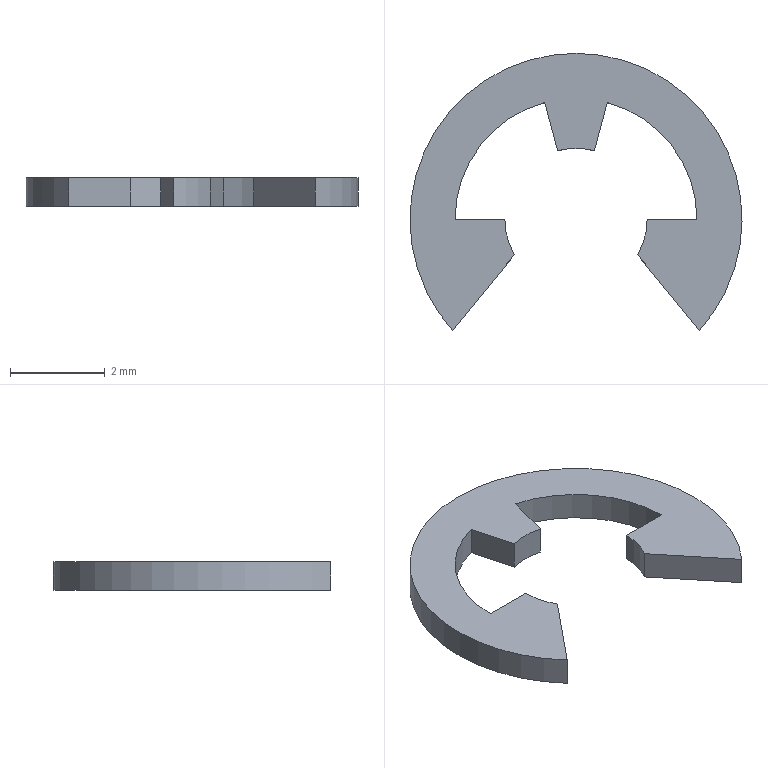Part | NX | 1 solid | 14 faces | box 7 x 5.843 x 0.6 mm | volume 10.111 mm3 | plane 8 | cylinder 6 | commonest cylinder face diameters 3 x3 5.1 x2 7 x1
STEP:
#1=CARTESIAN_POINT('',(2.6,-2.343,-0.3));
#2=VERTEX_POINT('',#1);
#3=CARTESIAN_POINT('',(-2.6,-2.343,-0.3));
#4=VERTEX_POINT('',#3);
#5=CARTESIAN_POINT('',(0.,0.,-0.3));
#6=DIRECTION('',(0.,0.,1.));
#7=DIRECTION('',(0.7429,-0.6694,0.));
#8=AXIS2_PLACEMENT_3D('',#5,#6,#7);
#9=CIRCLE('',#8,3.5);
#10=EDGE_CURVE('',#2,#4,#9,.T.);
#11=ORIENTED_EDGE('',*,*,#10,.T.);
#12=CARTESIAN_POINT('',(-2.6,-2.343,0.3));
#13=VERTEX_POINT('',#12);
#14=CARTESIAN_POINT('',(-2.6,-2.343,0.3));
#15=DIRECTION('',(0.,0.,-1.));
#16=VECTOR('',#15,1000.);
#17=LINE('',#14,#16);
#18=EDGE_CURVE('',#13,#4,#17,.T.);
#19=ORIENTED_EDGE('',*,*,#18,.F.);
#20=CARTESIAN_POINT('',(2.6,-2.343,0.3));
#21=VERTEX_POINT('',#20);
#22=CARTESIAN_POINT('',(0.,0.,0.3));
#23=DIRECTION('',(0.,0.,1.));
#24=DIRECTION('',(0.7429,-0.6694,0.));
#25=AXIS2_PLACEMENT_3D('',#22,#23,#24);
#26=CIRCLE('',#25,3.5);
#27=EDGE_CURVE('',#21,#13,#26,.T.);
#28=ORIENTED_EDGE('',*,*,#27,.F.);
#29=CARTESIAN_POINT('',(2.6,-2.343,0.3));
#30=DIRECTION('',(0.,0.,-1.));
#31=VECTOR('',#30,1000.);
#32=LINE('',#29,#31);
#33=EDGE_CURVE('',#21,#2,#32,.T.);
#34=ORIENTED_EDGE('',*,*,#33,.T.);
#35=EDGE_LOOP('',(#11,#19,#28,#34));
#36=FACE_BOUND('',#35,.T.);
#37=CARTESIAN_POINT('',(0.,0.,0.3));
#38=DIRECTION('',(0.,0.,1.));
#39=DIRECTION('',(0.7429,-0.6694,0.));
#40=AXIS2_PLACEMENT_3D('',#37,#38,#39);
#41=CYLINDRICAL_SURFACE('',#40,3.5);
#42=ADVANCED_FACE('',(#36),#41,.T.);
#43=CARTESIAN_POINT('',(-1.3,-0.7483,-0.3));
#44=VERTEX_POINT('',#43);
#45=CARTESIAN_POINT('',(-2.6,-2.343,-0.3));
#46=DIRECTION('',(0.6318,0.7751,0.));
#47=VECTOR('',#46,1000.);
#48=LINE('',#45,#47);
#49=EDGE_CURVE('',#4,#44,#48,.T.);
#50=ORIENTED_EDGE('',*,*,#49,.T.);
#51=CARTESIAN_POINT('',(-1.3,-0.7483,0.3));
#52=VERTEX_POINT('',#51);
#53=CARTESIAN_POINT('',(-1.3,-0.7483,0.3));
#54=DIRECTION('',(0.,0.,-1.));
#55=VECTOR('',#54,1000.);
#56=LINE('',#53,#55);
#57=EDGE_CURVE('',#52,#44,#56,.T.);
#58=ORIENTED_EDGE('',*,*,#57,.F.);
#59=CARTESIAN_POINT('',(-2.6,-2.343,0.3));
#60=DIRECTION('',(0.6318,0.7751,0.));
#61=VECTOR('',#60,1000.);
#62=LINE('',#59,#61);
#63=EDGE_CURVE('',#13,#52,#62,.T.);
#64=ORIENTED_EDGE('',*,*,#63,.F.);
#65=ORIENTED_EDGE('',*,*,#18,.T.);
#66=EDGE_LOOP('',(#50,#58,#64,#65));
#67=FACE_BOUND('',#66,.T.);
#68=CARTESIAN_POINT('',(-2.6,-2.343,0.3));
#69=DIRECTION('',(0.7751,-0.6318,0.));
#70=DIRECTION('',(0.,0.,-1.));
#71=AXIS2_PLACEMENT_3D('',#68,#69,#70);
#72=PLANE('',#71);
#73=ADVANCED_FACE('',(#67),#72,.T.);
#74=CARTESIAN_POINT('',(-1.5,0.,-0.3));
#75=VERTEX_POINT('',#74);
#76=CARTESIAN_POINT('',(0.,0.,-0.3));
#77=DIRECTION('',(0.,0.,-1.));
#78=DIRECTION('',(-0.8667,-0.4989,0.));
#79=AXIS2_PLACEMENT_3D('',#76,#77,#78);
#80=CIRCLE('',#79,1.5);
#81=EDGE_CURVE('',#44,#75,#80,.T.);
#82=ORIENTED_EDGE('',*,*,#81,.T.);
#83=CARTESIAN_POINT('',(-1.5,0.,0.3));
#84=VERTEX_POINT('',#83);
#85=CARTESIAN_POINT('',(-1.5,0.,0.3));
#86=DIRECTION('',(0.,0.,-1.));
#87=VECTOR('',#86,1000.);
#88=LINE('',#85,#87);
#89=EDGE_CURVE('',#84,#75,#88,.T.);
#90=ORIENTED_EDGE('',*,*,#89,.F.);
#91=CARTESIAN_POINT('',(0.,0.,0.3));
#92=DIRECTION('',(0.,0.,-1.));
#93=DIRECTION('',(-0.8667,-0.4989,0.));
#94=AXIS2_PLACEMENT_3D('',#91,#92,#93);
#95=CIRCLE('',#94,1.5);
#96=EDGE_CURVE('',#52,#84,#95,.T.);
#97=ORIENTED_EDGE('',*,*,#96,.F.);
#98=ORIENTED_EDGE('',*,*,#57,.T.);
#99=EDGE_LOOP('',(#82,#90,#97,#98));
#100=FACE_BOUND('',#99,.T.);
#101=CARTESIAN_POINT('',(0.,0.,0.3));
#102=DIRECTION('',(0.,0.,1.));
#103=DIRECTION('',(-0.8667,-0.4989,0.));
#104=AXIS2_PLACEMENT_3D('',#101,#102,#103);
#105=CYLINDRICAL_SURFACE('',#104,1.5);
#106=ADVANCED_FACE('',(#100),#105,.F.);
#107=CARTESIAN_POINT('',(-2.55,0.,-0.3));
#108=VERTEX_POINT('',#107);
#109=CARTESIAN_POINT('',(-1.5,0.,-0.3));
#110=DIRECTION('',(-1.,0.,0.));
#111=VECTOR('',#110,1000.);
#112=LINE('',#109,#111);
#113=EDGE_CURVE('',#75,#108,#112,.T.);
#114=ORIENTED_EDGE('',*,*,#113,.T.);
#115=CARTESIAN_POINT('',(-2.55,0.,0.3));
#116=VERTEX_POINT('',#115);
#117=CARTESIAN_POINT('',(-2.55,0.,0.3));
#118=DIRECTION('',(0.,0.,-1.));
#119=VECTOR('',#118,1000.);
#120=LINE('',#117,#119);
#121=EDGE_CURVE('',#116,#108,#120,.T.);
#122=ORIENTED_EDGE('',*,*,#121,.F.);
#123=CARTESIAN_POINT('',(-1.5,0.,0.3));
#124=DIRECTION('',(-1.,0.,0.));
#125=VECTOR('',#124,1000.);
#126=LINE('',#123,#125);
#127=EDGE_CURVE('',#84,#116,#126,.T.);
#128=ORIENTED_EDGE('',*,*,#127,.F.);
#129=ORIENTED_EDGE('',*,*,#89,.T.);
#130=EDGE_LOOP('',(#114,#122,#128,#129));
#131=FACE_BOUND('',#130,.T.);
#132=CARTESIAN_POINT('',(-1.5,0.,0.3));
#133=DIRECTION('',(0.,1.,0.));
#134=DIRECTION('',(1.,0.,0.));
#135=AXIS2_PLACEMENT_3D('',#132,#133,#134);
#136=PLANE('',#135);
#137=ADVANCED_FACE('',(#131),#136,.T.);
#138=CARTESIAN_POINT('',(-0.66,2.463,-0.3));
#139=VERTEX_POINT('',#138);
#140=CARTESIAN_POINT('',(0.,0.,-0.3));
#141=DIRECTION('',(0.,0.,-1.));
#142=DIRECTION('',(-1.,0.,0.));
#143=AXIS2_PLACEMENT_3D('',#140,#141,#142);
#144=CIRCLE('',#143,2.55);
#145=EDGE_CURVE('',#108,#139,#144,.T.);
#146=ORIENTED_EDGE('',*,*,#145,.T.);
#147=CARTESIAN_POINT('',(-0.66,2.463,0.3));
#148=VERTEX_POINT('',#147);
#149=CARTESIAN_POINT('',(-0.66,2.463,0.3));
#150=DIRECTION('',(0.,0.,-1.));
#151=VECTOR('',#150,1000.);
#152=LINE('',#149,#151);
#153=EDGE_CURVE('',#148,#139,#152,.T.);
#154=ORIENTED_EDGE('',*,*,#153,.F.);
#155=CARTESIAN_POINT('',(0.,0.,0.3));
#156=DIRECTION('',(0.,0.,-1.));
#157=DIRECTION('',(-1.,0.,0.));
#158=AXIS2_PLACEMENT_3D('',#155,#156,#157);
#159=CIRCLE('',#158,2.55);
#160=EDGE_CURVE('',#116,#148,#159,.T.);
#161=ORIENTED_EDGE('',*,*,#160,.F.);
#162=ORIENTED_EDGE('',*,*,#121,.T.);
#163=EDGE_LOOP('',(#146,#154,#161,#162));
#164=FACE_BOUND('',#163,.T.);
#165=CARTESIAN_POINT('',(0.,0.,0.3));
#166=DIRECTION('',(0.,0.,1.));
#167=DIRECTION('',(-1.,0.,0.));
#168=AXIS2_PLACEMENT_3D('',#165,#166,#167);
#169=CYLINDRICAL_SURFACE('',#168,2.55);
#170=ADVANCED_FACE('',(#164),#169,.F.);
#171=CARTESIAN_POINT('',(-0.3882,1.449,-0.3));
#172=VERTEX_POINT('',#171);
#173=CARTESIAN_POINT('',(-0.66,2.463,-0.3));
#174=DIRECTION('',(0.2588,-0.9659,0.));
#175=VECTOR('',#174,1000.);
#176=LINE('',#173,#175);
#177=EDGE_CURVE('',#139,#172,#176,.T.);
#178=ORIENTED_EDGE('',*,*,#177,.T.);
#179=CARTESIAN_POINT('',(-0.3882,1.449,0.3));
#180=VERTEX_POINT('',#179);
#181=CARTESIAN_POINT('',(-0.3882,1.449,0.3));
#182=DIRECTION('',(0.,0.,-1.));
#183=VECTOR('',#182,1000.);
#184=LINE('',#181,#183);
#185=EDGE_CURVE('',#180,#172,#184,.T.);
#186=ORIENTED_EDGE('',*,*,#185,.F.);
#187=CARTESIAN_POINT('',(-0.66,2.463,0.3));
#188=DIRECTION('',(0.2588,-0.9659,0.));
#189=VECTOR('',#188,1000.);
#190=LINE('',#187,#189);
#191=EDGE_CURVE('',#148,#180,#190,.T.);
#192=ORIENTED_EDGE('',*,*,#191,.F.);
#193=ORIENTED_EDGE('',*,*,#153,.T.);
#194=EDGE_LOOP('',(#178,#186,#192,#193));
#195=FACE_BOUND('',#194,.T.);
#196=CARTESIAN_POINT('',(-0.66,2.463,0.3));
#197=DIRECTION('',(-0.9659,-0.2588,0.));
#198=DIRECTION('',(-0.2588,0.9659,0.));
#199=AXIS2_PLACEMENT_3D('',#196,#197,#198);
#200=PLANE('',#199);
#201=ADVANCED_FACE('',(#195),#200,.T.);
#202=CARTESIAN_POINT('',(0.3882,1.449,-0.3));
#203=VERTEX_POINT('',#202);
#204=CARTESIAN_POINT('',(0.,0.,-0.3));
#205=DIRECTION('',(0.,0.,-1.));
#206=DIRECTION('',(-0.2588,0.9659,0.));
#207=AXIS2_PLACEMENT_3D('',#204,#205,#206);
#208=CIRCLE('',#207,1.5);
#209=EDGE_CURVE('',#172,#203,#208,.T.);
#210=ORIENTED_EDGE('',*,*,#209,.T.);
#211=CARTESIAN_POINT('',(0.3882,1.449,0.3));
#212=VERTEX_POINT('',#211);
#213=CARTESIAN_POINT('',(0.3882,1.449,0.3));
#214=DIRECTION('',(0.,0.,-1.));
#215=VECTOR('',#214,1000.);
#216=LINE('',#213,#215);
#217=EDGE_CURVE('',#212,#203,#216,.T.);
#218=ORIENTED_EDGE('',*,*,#217,.F.);
#219=CARTESIAN_POINT('',(0.,0.,0.3));
#220=DIRECTION('',(0.,0.,-1.));
#221=DIRECTION('',(-0.2588,0.9659,0.));
#222=AXIS2_PLACEMENT_3D('',#219,#220,#221);
#223=CIRCLE('',#222,1.5);
#224=EDGE_CURVE('',#180,#212,#223,.T.);
#225=ORIENTED_EDGE('',*,*,#224,.F.);
#226=ORIENTED_EDGE('',*,*,#185,.T.);
#227=EDGE_LOOP('',(#210,#218,#225,#226));
#228=FACE_BOUND('',#227,.T.);
#229=CARTESIAN_POINT('',(0.,0.,0.3));
#230=DIRECTION('',(0.,0.,1.));
#231=DIRECTION('',(-0.2588,0.9659,0.));
#232=AXIS2_PLACEMENT_3D('',#229,#230,#231);
#233=CYLINDRICAL_SURFACE('',#232,1.5);
#234=ADVANCED_FACE('',(#228),#233,.F.);
#235=CARTESIAN_POINT('',(0.66,2.463,-0.3));
#236=VERTEX_POINT('',#235);
#237=CARTESIAN_POINT('',(0.3882,1.449,-0.3));
#238=DIRECTION('',(0.2588,0.9659,0.));
#239=VECTOR('',#238,1000.);
#240=LINE('',#237,#239);
#241=EDGE_CURVE('',#203,#236,#240,.T.);
#242=ORIENTED_EDGE('',*,*,#241,.T.);
#243=CARTESIAN_POINT('',(0.66,2.463,0.3));
#244=VERTEX_POINT('',#243);
#245=CARTESIAN_POINT('',(0.66,2.463,0.3));
#246=DIRECTION('',(0.,0.,-1.));
#247=VECTOR('',#246,1000.);
#248=LINE('',#245,#247);
#249=EDGE_CURVE('',#244,#236,#248,.T.);
#250=ORIENTED_EDGE('',*,*,#249,.F.);
#251=CARTESIAN_POINT('',(0.3882,1.449,0.3));
#252=DIRECTION('',(0.2588,0.9659,0.));
#253=VECTOR('',#252,1000.);
#254=LINE('',#251,#253);
#255=EDGE_CURVE('',#212,#244,#254,.T.);
#256=ORIENTED_EDGE('',*,*,#255,.F.);
#257=ORIENTED_EDGE('',*,*,#217,.T.);
#258=EDGE_LOOP('',(#242,#250,#256,#257));
#259=FACE_BOUND('',#258,.T.);
#260=CARTESIAN_POINT('',(0.3882,1.449,0.3));
#261=DIRECTION('',(0.9659,-0.2588,0.));
#262=DIRECTION('',(0.,0.,-1.));
#263=AXIS2_PLACEMENT_3D('',#260,#261,#262);
#264=PLANE('',#263);
#265=ADVANCED_FACE('',(#259),#264,.T.);
#266=CARTESIAN_POINT('',(2.55,0.,-0.3));
#267=VERTEX_POINT('',#266);
#268=CARTESIAN_POINT('',(0.,0.,-0.3));
#269=DIRECTION('',(0.,0.,-1.));
#270=DIRECTION('',(0.2588,0.9659,0.));
#271=AXIS2_PLACEMENT_3D('',#268,#269,#270);
#272=CIRCLE('',#271,2.55);
#273=EDGE_CURVE('',#236,#267,#272,.T.);
#274=ORIENTED_EDGE('',*,*,#273,.T.);
#275=CARTESIAN_POINT('',(2.55,0.,0.3));
#276=VERTEX_POINT('',#275);
#277=CARTESIAN_POINT('',(2.55,0.,0.3));
#278=DIRECTION('',(0.,0.,-1.));
#279=VECTOR('',#278,1000.);
#280=LINE('',#277,#279);
#281=EDGE_CURVE('',#276,#267,#280,.T.);
#282=ORIENTED_EDGE('',*,*,#281,.F.);
#283=CARTESIAN_POINT('',(0.,0.,0.3));
#284=DIRECTION('',(0.,0.,-1.));
#285=DIRECTION('',(0.2588,0.9659,0.));
#286=AXIS2_PLACEMENT_3D('',#283,#284,#285);
#287=CIRCLE('',#286,2.55);
#288=EDGE_CURVE('',#244,#276,#287,.T.);
#289=ORIENTED_EDGE('',*,*,#288,.F.);
#290=ORIENTED_EDGE('',*,*,#249,.T.);
#291=EDGE_LOOP('',(#274,#282,#289,#290));
#292=FACE_BOUND('',#291,.T.);
#293=CARTESIAN_POINT('',(0.,0.,0.3));
#294=DIRECTION('',(0.,0.,1.));
#295=DIRECTION('',(0.2588,0.9659,0.));
#296=AXIS2_PLACEMENT_3D('',#293,#294,#295);
#297=CYLINDRICAL_SURFACE('',#296,2.55);
#298=ADVANCED_FACE('',(#292),#297,.F.);
#299=CARTESIAN_POINT('',(1.5,0.,-0.3));
#300=VERTEX_POINT('',#299);
#301=CARTESIAN_POINT('',(2.55,0.,-0.3));
#302=DIRECTION('',(-1.,0.,0.));
#303=VECTOR('',#302,1000.);
#304=LINE('',#301,#303);
#305=EDGE_CURVE('',#267,#300,#304,.T.);
#306=ORIENTED_EDGE('',*,*,#305,.T.);
#307=CARTESIAN_POINT('',(1.5,0.,0.3));
#308=VERTEX_POINT('',#307);
#309=CARTESIAN_POINT('',(1.5,0.,0.3));
#310=DIRECTION('',(0.,0.,-1.));
#311=VECTOR('',#310,1000.);
#312=LINE('',#309,#311);
#313=EDGE_CURVE('',#308,#300,#312,.T.);
#314=ORIENTED_EDGE('',*,*,#313,.F.);
#315=CARTESIAN_POINT('',(2.55,0.,0.3));
#316=DIRECTION('',(-1.,0.,0.));
#317=VECTOR('',#316,1000.);
#318=LINE('',#315,#317);
#319=EDGE_CURVE('',#276,#308,#318,.T.);
#320=ORIENTED_EDGE('',*,*,#319,.F.);
#321=ORIENTED_EDGE('',*,*,#281,.T.);
#322=EDGE_LOOP('',(#306,#314,#320,#321));
#323=FACE_BOUND('',#322,.T.);
#324=CARTESIAN_POINT('',(2.55,0.,0.3));
#325=DIRECTION('',(0.,1.,0.));
#326=DIRECTION('',(1.,0.,0.));
#327=AXIS2_PLACEMENT_3D('',#324,#325,#326);
#328=PLANE('',#327);
#329=ADVANCED_FACE('',(#323),#328,.T.);
#330=CARTESIAN_POINT('',(1.3,-0.7483,-0.3));
#331=VERTEX_POINT('',#330);
#332=CARTESIAN_POINT('',(0.,0.,-0.3));
#333=DIRECTION('',(0.,0.,-1.));
#334=DIRECTION('',(1.,0.,0.));
#335=AXIS2_PLACEMENT_3D('',#332,#333,#334);
#336=CIRCLE('',#335,1.5);
#337=EDGE_CURVE('',#300,#331,#336,.T.);
#338=ORIENTED_EDGE('',*,*,#337,.T.);
#339=CARTESIAN_POINT('',(1.3,-0.7483,0.3));
#340=VERTEX_POINT('',#339);
#341=CARTESIAN_POINT('',(1.3,-0.7483,0.3));
#342=DIRECTION('',(0.,0.,-1.));
#343=VECTOR('',#342,1000.);
#344=LINE('',#341,#343);
#345=EDGE_CURVE('',#340,#331,#344,.T.);
#346=ORIENTED_EDGE('',*,*,#345,.F.);
#347=CARTESIAN_POINT('',(0.,0.,0.3));
#348=DIRECTION('',(0.,0.,-1.));
#349=DIRECTION('',(1.,0.,0.));
#350=AXIS2_PLACEMENT_3D('',#347,#348,#349);
#351=CIRCLE('',#350,1.5);
#352=EDGE_CURVE('',#308,#340,#351,.T.);
#353=ORIENTED_EDGE('',*,*,#352,.F.);
#354=ORIENTED_EDGE('',*,*,#313,.T.);
#355=EDGE_LOOP('',(#338,#346,#353,#354));
#356=FACE_BOUND('',#355,.T.);
#357=CARTESIAN_POINT('',(0.,0.,0.3));
#358=DIRECTION('',(0.,0.,1.));
#359=DIRECTION('',(1.,0.,0.));
#360=AXIS2_PLACEMENT_3D('',#357,#358,#359);
#361=CYLINDRICAL_SURFACE('',#360,1.5);
#362=ADVANCED_FACE('',(#356),#361,.F.);
#363=CARTESIAN_POINT('',(1.3,-0.7483,-0.3));
#364=DIRECTION('',(0.6318,-0.7751,0.));
#365=VECTOR('',#364,1000.);
#366=LINE('',#363,#365);
#367=EDGE_CURVE('',#331,#2,#366,.T.);
#368=ORIENTED_EDGE('',*,*,#367,.T.);
#369=ORIENTED_EDGE('',*,*,#33,.F.);
#370=CARTESIAN_POINT('',(1.3,-0.7483,0.3));
#371=DIRECTION('',(0.6318,-0.7751,0.));
#372=VECTOR('',#371,1000.);
#373=LINE('',#370,#372);
#374=EDGE_CURVE('',#340,#21,#373,.T.);
#375=ORIENTED_EDGE('',*,*,#374,.F.);
#376=ORIENTED_EDGE('',*,*,#345,.T.);
#377=EDGE_LOOP('',(#368,#369,#375,#376));
#378=FACE_BOUND('',#377,.T.);
#379=CARTESIAN_POINT('',(1.3,-0.7483,0.3));
#380=DIRECTION('',(-0.7751,-0.6318,0.));
#381=DIRECTION('',(-0.6318,0.7751,0.));
#382=AXIS2_PLACEMENT_3D('',#379,#380,#381);
#383=PLANE('',#382);
#384=ADVANCED_FACE('',(#378),#383,.T.);
#385=ORIENTED_EDGE('',*,*,#27,.T.);
#386=ORIENTED_EDGE('',*,*,#63,.T.);
#387=ORIENTED_EDGE('',*,*,#96,.T.);
#388=ORIENTED_EDGE('',*,*,#127,.T.);
#389=ORIENTED_EDGE('',*,*,#160,.T.);
#390=ORIENTED_EDGE('',*,*,#191,.T.);
#391=ORIENTED_EDGE('',*,*,#224,.T.);
#392=ORIENTED_EDGE('',*,*,#255,.T.);
#393=ORIENTED_EDGE('',*,*,#288,.T.);
#394=ORIENTED_EDGE('',*,*,#319,.T.);
#395=ORIENTED_EDGE('',*,*,#352,.T.);
#396=ORIENTED_EDGE('',*,*,#374,.T.);
#397=EDGE_LOOP('',(#385,#386,#387,#388,#389,#390,#391,#392,#393,#394,#395,#396));
#398=FACE_BOUND('',#397,.T.);
#399=CARTESIAN_POINT('',(0.,0.,0.3));
#400=DIRECTION('',(0.,0.,1.));
#401=DIRECTION('',(1.,0.,0.));
#402=AXIS2_PLACEMENT_3D('',#399,#400,#401);
#403=PLANE('',#402);
#404=ADVANCED_FACE('',(#398),#403,.T.);
#405=ORIENTED_EDGE('',*,*,#49,.F.);
#406=ORIENTED_EDGE('',*,*,#10,.F.);
#407=ORIENTED_EDGE('',*,*,#367,.F.);
#408=ORIENTED_EDGE('',*,*,#337,.F.);
#409=ORIENTED_EDGE('',*,*,#305,.F.);
#410=ORIENTED_EDGE('',*,*,#273,.F.);
#411=ORIENTED_EDGE('',*,*,#241,.F.);
#412=ORIENTED_EDGE('',*,*,#209,.F.);
#413=ORIENTED_EDGE('',*,*,#177,.F.);
#414=ORIENTED_EDGE('',*,*,#145,.F.);
#415=ORIENTED_EDGE('',*,*,#113,.F.);
#416=ORIENTED_EDGE('',*,*,#81,.F.);
#417=EDGE_LOOP('',(#405,#406,#407,#408,#409,#410,#411,#412,#413,#414,#415,#416));
#418=FACE_BOUND('',#417,.T.);
#419=CARTESIAN_POINT('',(0.,0.,-0.3));
#420=DIRECTION('',(0.,0.,1.));
#421=DIRECTION('',(1.,0.,0.));
#422=AXIS2_PLACEMENT_3D('',#419,#420,#421);
#423=PLANE('',#422);
#424=ADVANCED_FACE('',(#418),#423,.F.);
#425=CLOSED_SHELL('',(#42,#73,#106,#137,#170,#201,#234,#265,#298,#329,#362,#384,#404,#424));
#426=MANIFOLD_SOLID_BREP('',#425);
#427=(LENGTH_UNIT()NAMED_UNIT(*)SI_UNIT(.MILLI.,.METRE.));
#428=UNCERTAINTY_MEASURE_WITH_UNIT(LENGTH_MEASURE(0.00001),#427,'','');
#429=(NAMED_UNIT(*)PLANE_ANGLE_UNIT()SI_UNIT($,.RADIAN.));
#430=(NAMED_UNIT(*)SI_UNIT($,.STERADIAN.)SOLID_ANGLE_UNIT());
#431=(GEOMETRIC_REPRESENTATION_CONTEXT(3)GLOBAL_UNCERTAINTY_ASSIGNED_CONTEXT((#428))GLOBAL_UNIT_ASSIGNED_CONTEXT((#427,#429,#430))REPRESENTATION_CONTEXT('',''));
#432=ADVANCED_BREP_SHAPE_REPRESENTATION('',(#426),#431);